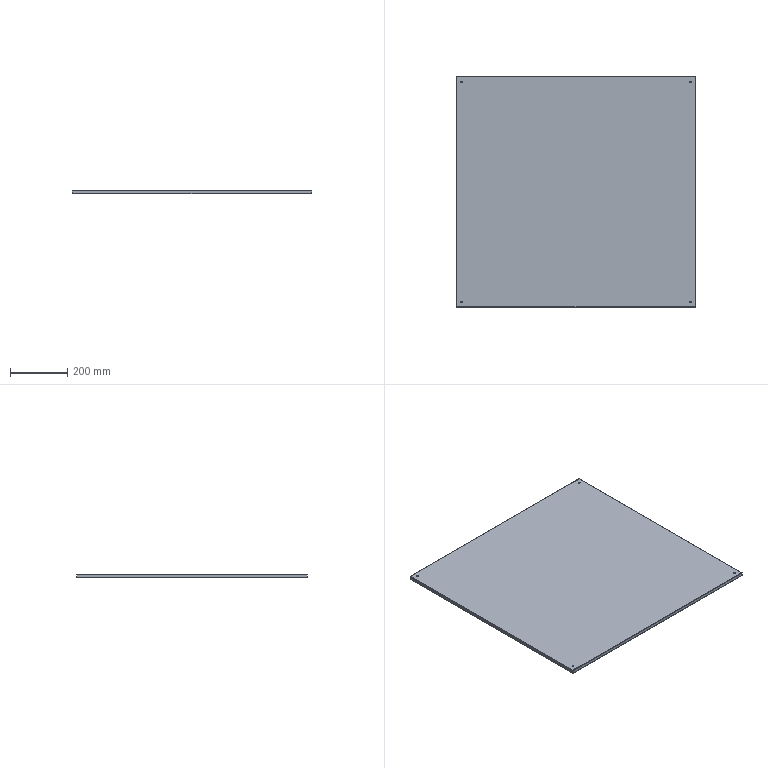Part | SolidWorks | features EdgeFlange 2, FlatPattern 1, ICE 1, SMBaseFlange 1, SheetMetal 1 | 1 solid | 78 faces | box 837 x 807 x 13 mm | volume 1107218 mm3 | plane 38 | cylinder 24 | spline 16 | commonest cylinder face diameters 0.2 x8 3.2 x8 6.5 x8